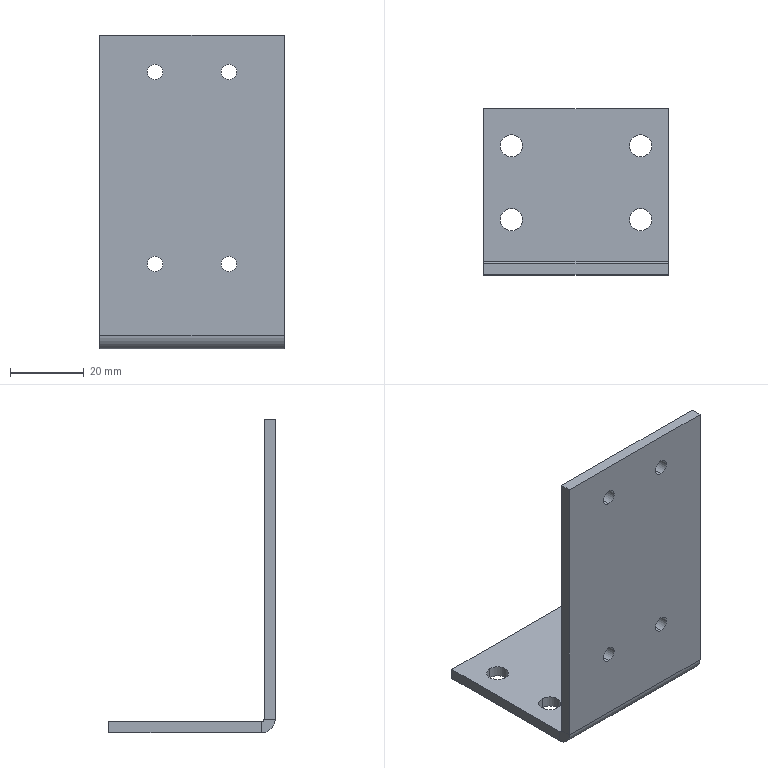Part | STEP file | 3038 drag chain bracket | 1 solid | 30 faces | box 50 x 45 x 85 mm | volume 18400 mm3 | cylinder 18 | plane 12 | commonest cylinder face diameters 4.2 x8 6 x8 1.473 x1 7.473 x1